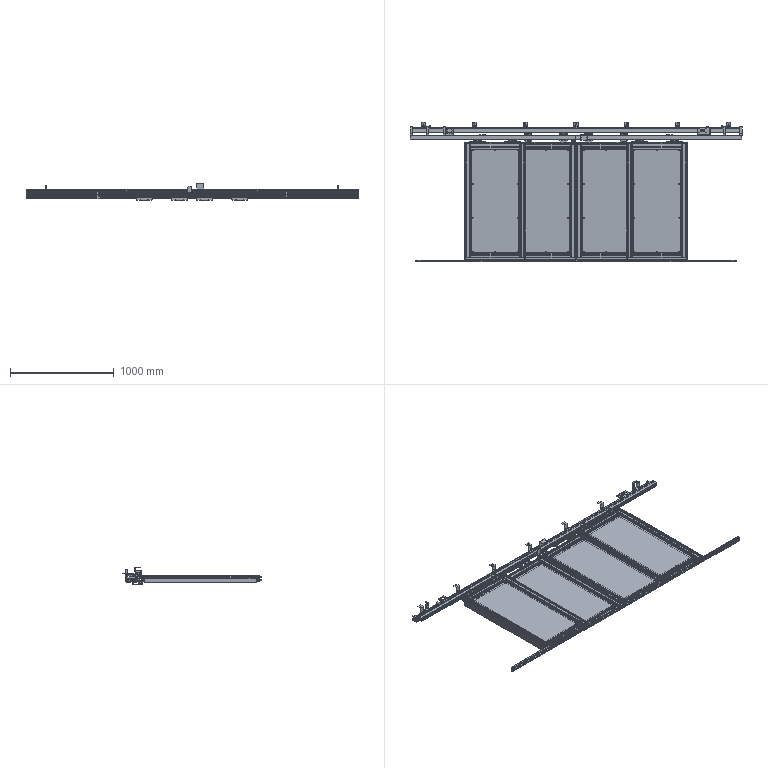Part | NX | features BREP 41 | 121 solids | 5894 faces | volume 18737251 mm3 | plane 2756 | cylinder 2356 | torus 480 | cone 232 | spline 64 | sphere 6 | commonest cylinder face diameters 4 x273 5 x176 4.2 x160 7 x158 12 x158 3.3 x144